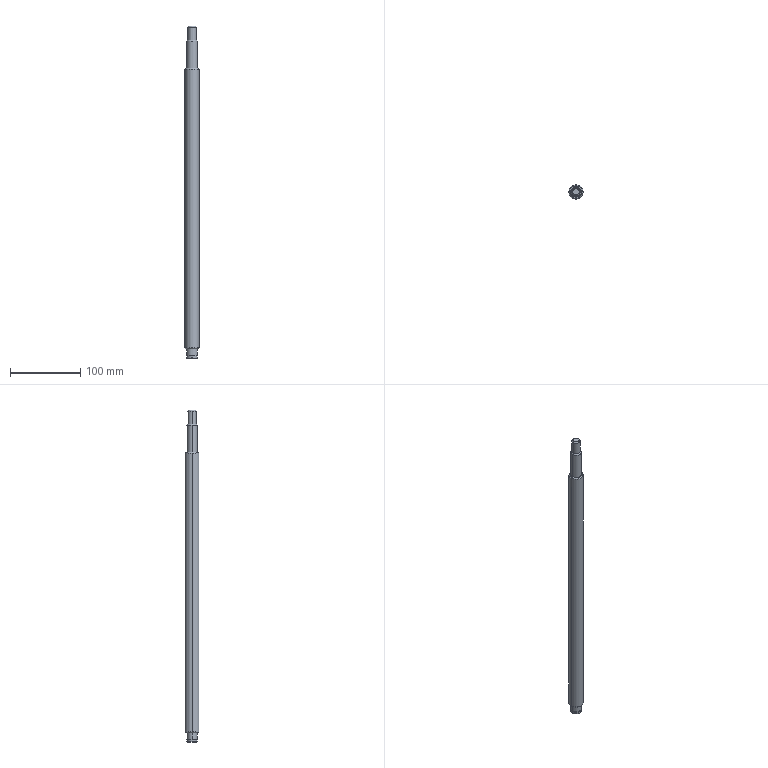Part | STEP file | 1 solid | 28 faces | box 20 x 20 x 472 mm | volume 136774 mm3 | cylinder 12 | cone 10 | plane 6 | commonest cylinder face diameters 15 x6 12 x2 14.3 x2 20 x2